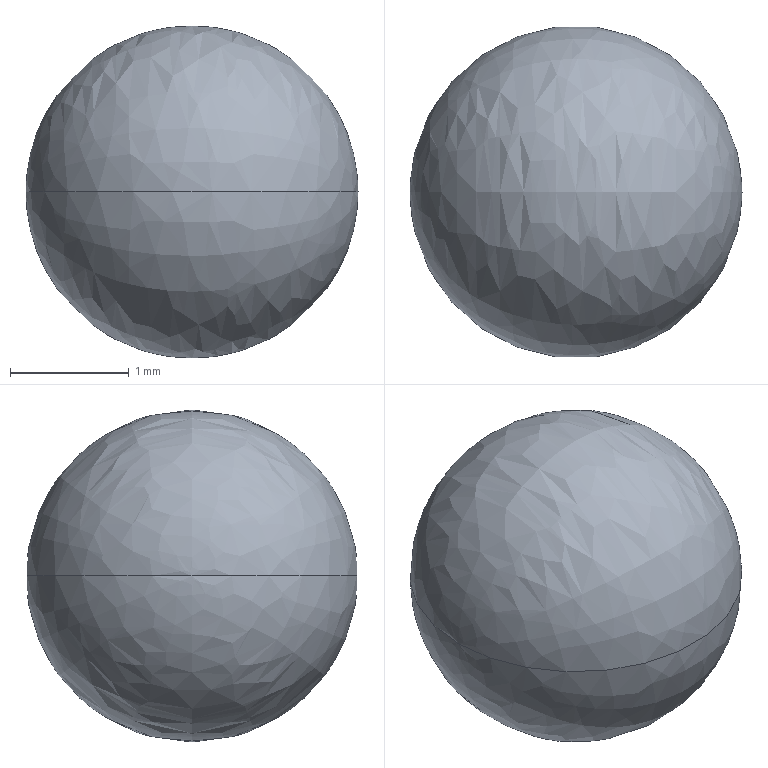Part | SolidWorks | features BaseBody 1 | 1 solid | 2 faces | volume 11.494 mm3 | spline 2
STEP:
#1=CARTESIAN_POINT('',(1.4,0.,0.));
#2=VERTEX_POINT('',#1);
#3=CARTESIAN_POINT('',(-1.4,0.,0.));
#4=VERTEX_POINT('',#3);
#5=CARTESIAN_POINT('',(0.,0.,0.));
#6=DIRECTION('',(0.,0.,1.));
#7=DIRECTION('',(1.,0.,0.));
#8=AXIS2_PLACEMENT_3D('',#5,#6,#7);
#9=CIRCLE('',#8,1.4);
#10=EDGE_CURVE('',#2,#4,#9,.T.);
#11=ORIENTED_EDGE('',*,*,#10,.F.);
#12=CARTESIAN_POINT('',(0.,0.,0.));
#13=DIRECTION('',(0.,0.,-1.));
#14=DIRECTION('',(1.,0.,0.));
#15=AXIS2_PLACEMENT_3D('',#12,#13,#14);
#16=CIRCLE('',#15,1.4);
#17=EDGE_CURVE('',#2,#4,#16,.T.);
#18=ORIENTED_EDGE('',*,*,#17,.T.);
#19=EDGE_LOOP('',(#11,#18));
#20=FACE_OUTER_BOUND('',#19,.T.);
#21=CARTESIAN_POINT('',(1.4,0.,0.));
#22=CARTESIAN_POINT('',(1.4,0.,0.));
#23=CARTESIAN_POINT('',(1.4,0.,0.));
#24=CARTESIAN_POINT('',(1.4,0.,0.));
#25=CARTESIAN_POINT('',(1.4,-2.8,0.));
#26=CARTESIAN_POINT('',(1.4,-2.8,-5.6));
#27=CARTESIAN_POINT('',(1.4,2.8,-5.6));
#28=CARTESIAN_POINT('',(1.4,2.8,0.));
#29=CARTESIAN_POINT('',(-1.4,-2.8,0.));
#30=CARTESIAN_POINT('',(-1.4,-2.8,-5.6));
#31=CARTESIAN_POINT('',(-1.4,2.8,-5.6));
#32=CARTESIAN_POINT('',(-1.4,2.8,0.));
#33=CARTESIAN_POINT('',(-1.4,0.,0.));
#34=CARTESIAN_POINT('',(-1.4,0.,0.));
#35=CARTESIAN_POINT('',(-1.4,0.,0.));
#36=CARTESIAN_POINT('',(-1.4,0.,0.));
#37=(BOUNDED_SURFACE()B_SPLINE_SURFACE(3,3,((#21,#22,#23,#24),(#25,#26,#27,#28),(#29,#30,#31,#32),(#33,#34,#35,#36)),.UNSPECIFIED.,.F.,.F.,.F.)B_SPLINE_SURFACE_WITH_KNOTS((4,4),(4,4),(0.,1.),(0.,1.),.UNSPECIFIED.)GEOMETRIC_REPRESENTATION_ITEM()RATIONAL_B_SPLINE_SURFACE(((1.,0.3333,0.3333,1.),(0.3333,0.1111,0.1111,0.3333),(0.3333,0.1111,0.1111,0.3333),(1.,0.3333,0.3333,1.)))REPRESENTATION_ITEM('')SURFACE());
#38=ADVANCED_FACE('',(#20),#37,.T.);
#39=ORIENTED_EDGE('',*,*,#17,.F.);
#40=ORIENTED_EDGE('',*,*,#10,.T.);
#41=EDGE_LOOP('',(#39,#40));
#42=FACE_OUTER_BOUND('',#41,.T.);
#43=CARTESIAN_POINT('',(1.4,0.,0.));
#44=CARTESIAN_POINT('',(1.4,0.,0.));
#45=CARTESIAN_POINT('',(1.4,0.,0.));
#46=CARTESIAN_POINT('',(1.4,0.,0.));
#47=CARTESIAN_POINT('',(1.4,2.8,0.));
#48=CARTESIAN_POINT('',(1.4,2.8,5.6));
#49=CARTESIAN_POINT('',(1.4,-2.8,5.6));
#50=CARTESIAN_POINT('',(1.4,-2.8,0.));
#51=CARTESIAN_POINT('',(-1.4,2.8,0.));
#52=CARTESIAN_POINT('',(-1.4,2.8,5.6));
#53=CARTESIAN_POINT('',(-1.4,-2.8,5.6));
#54=CARTESIAN_POINT('',(-1.4,-2.8,0.));
#55=CARTESIAN_POINT('',(-1.4,0.,0.));
#56=CARTESIAN_POINT('',(-1.4,0.,0.));
#57=CARTESIAN_POINT('',(-1.4,0.,0.));
#58=CARTESIAN_POINT('',(-1.4,0.,0.));
#59=(BOUNDED_SURFACE()B_SPLINE_SURFACE(3,3,((#43,#44,#45,#46),(#47,#48,#49,#50),(#51,#52,#53,#54),(#55,#56,#57,#58)),.UNSPECIFIED.,.F.,.F.,.F.)B_SPLINE_SURFACE_WITH_KNOTS((4,4),(4,4),(0.,1.),(0.,1.),.UNSPECIFIED.)GEOMETRIC_REPRESENTATION_ITEM()RATIONAL_B_SPLINE_SURFACE(((1.,0.3333,0.3333,1.),(0.3333,0.1111,0.1111,0.3333),(0.3333,0.1111,0.1111,0.3333),(1.,0.3333,0.3333,1.)))REPRESENTATION_ITEM('')SURFACE());
#60=ADVANCED_FACE('',(#42),#59,.T.);
#61=CLOSED_SHELL('',(#38,#60));
#62=MANIFOLD_SOLID_BREP('',#61);
#63=CARTESIAN_POINT('',(0.,0.,0.));
#64=DIRECTION('',(0.,0.,1.));
#65=DIRECTION('',(1.,0.,0.));
#66=AXIS2_PLACEMENT_3D('',#63,#64,#65);
#67=(LENGTH_UNIT()NAMED_UNIT(*)SI_UNIT(.MILLI.,.METRE.));
#68=UNCERTAINTY_MEASURE_WITH_UNIT(LENGTH_MEASURE(0.00001),#67,'','');
#69=(NAMED_UNIT(*)PLANE_ANGLE_UNIT()SI_UNIT($,.RADIAN.));
#70=(NAMED_UNIT(*)SI_UNIT($,.STERADIAN.)SOLID_ANGLE_UNIT());
#71=(GEOMETRIC_REPRESENTATION_CONTEXT(3)GLOBAL_UNCERTAINTY_ASSIGNED_CONTEXT((#68))GLOBAL_UNIT_ASSIGNED_CONTEXT((#67,#69,#70))REPRESENTATION_CONTEXT('',''));
#72=ADVANCED_BREP_SHAPE_REPRESENTATION('',(#62,#66),#71);